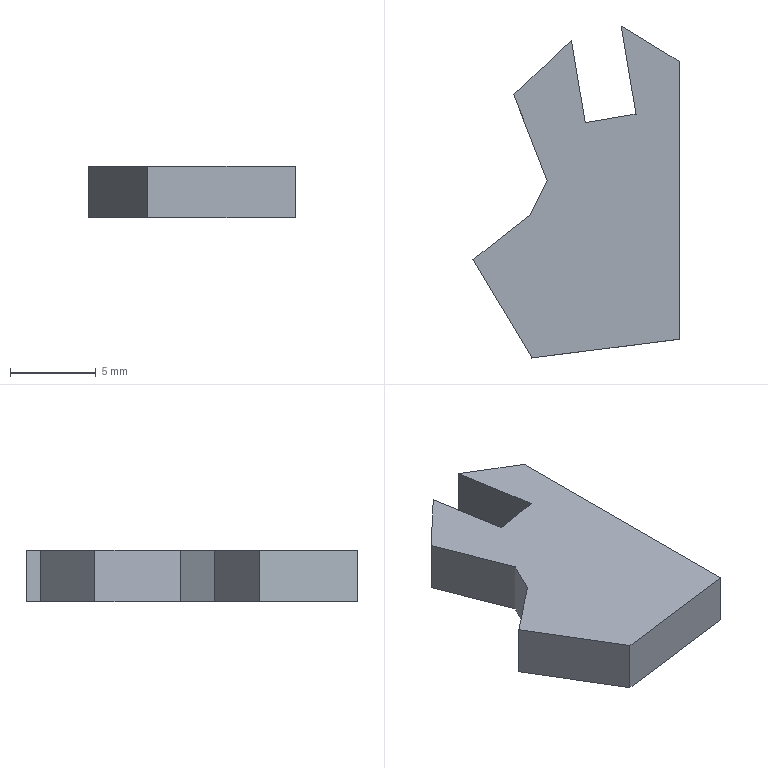Part | SolidWorks | features BaseBody 1 | 1 solid | 13 faces | box 12.009 x 19.33 x 3 mm | volume 454.514 mm3 | spline 7 | plane 6
STEP:
#1=CARTESIAN_POINT('',(-8.721,-24.916,-1.5));
#2=VERTEX_POINT('',#1);
#3=CARTESIAN_POINT('',(-0.1475,-23.826,-1.5));
#4=VERTEX_POINT('',#3);
#5=CARTESIAN_POINT('',(-8.721,-24.916,-1.5));
#6=CARTESIAN_POINT('',(-5.863,-24.552,-1.5));
#7=CARTESIAN_POINT('',(-3.006,-24.188,-1.5));
#8=CARTESIAN_POINT('',(-0.1475,-23.826,-1.5));
#9=B_SPLINE_CURVE_WITH_KNOTS('',3,(#5,#6,#7,#8),.UNSPECIFIED.,.F.,.F.,(4,4),(0.,0.05556),.UNSPECIFIED.);
#10=EDGE_CURVE('',#2,#4,#9,.T.);
#11=ORIENTED_EDGE('',*,*,#10,.F.);
#12=CARTESIAN_POINT('',(-12.156,-19.203,-1.5));
#13=VERTEX_POINT('',#12);
#14=CARTESIAN_POINT('',(-12.156,-19.203,-1.5));
#15=CARTESIAN_POINT('',(-11.011,-21.106,-1.5));
#16=CARTESIAN_POINT('',(-9.865,-23.01,-1.5));
#17=CARTESIAN_POINT('',(-8.721,-24.916,-1.5));
#18=B_SPLINE_CURVE_WITH_KNOTS('',3,(#14,#15,#16,#17),.UNSPECIFIED.,.F.,.F.,(4,4),(0.05556,0.1111),.UNSPECIFIED.);
#19=EDGE_CURVE('',#13,#2,#18,.T.);
#20=ORIENTED_EDGE('',*,*,#19,.F.);
#21=CARTESIAN_POINT('',(-8.807,-16.561,-1.5));
#22=VERTEX_POINT('',#21);
#23=CARTESIAN_POINT('',(-8.807,-16.561,-1.5));
#24=CARTESIAN_POINT('',(-9.924,-17.443,-1.5));
#25=CARTESIAN_POINT('',(-11.04,-18.323,-1.5));
#26=CARTESIAN_POINT('',(-12.156,-19.203,-1.5));
#27=B_SPLINE_CURVE_WITH_KNOTS('',3,(#23,#24,#25,#26),.UNSPECIFIED.,.F.,.F.,(4,4),(0.1111,0.1667),.UNSPECIFIED.);
#28=EDGE_CURVE('',#22,#13,#27,.T.);
#29=ORIENTED_EDGE('',*,*,#28,.F.);
#30=CARTESIAN_POINT('',(-7.838,-14.581,-1.5));
#31=VERTEX_POINT('',#30);
#32=CARTESIAN_POINT('',(-7.838,-14.581,-1.5));
#33=CARTESIAN_POINT('',(-8.163,-15.241,-1.5));
#34=CARTESIAN_POINT('',(-8.485,-15.903,-1.5));
#35=CARTESIAN_POINT('',(-8.807,-16.561,-1.5));
#36=B_SPLINE_CURVE_WITH_KNOTS('',3,(#32,#33,#34,#35),.UNSPECIFIED.,.F.,.F.,(4,4),(0.1667,0.2222),.UNSPECIFIED.);
#37=EDGE_CURVE('',#31,#22,#36,.T.);
#38=ORIENTED_EDGE('',*,*,#37,.F.);
#39=CARTESIAN_POINT('',(-9.774,-9.593,-1.5));
#40=VERTEX_POINT('',#39);
#41=CARTESIAN_POINT('',(-9.774,-9.593,-1.5));
#42=CARTESIAN_POINT('',(-9.129,-11.256,-1.5));
#43=CARTESIAN_POINT('',(-8.485,-12.919,-1.5));
#44=CARTESIAN_POINT('',(-7.838,-14.581,-1.5));
#45=B_SPLINE_CURVE_WITH_KNOTS('',3,(#41,#42,#43,#44),.UNSPECIFIED.,.F.,.F.,(4,4),(0.2222,0.2778),.UNSPECIFIED.);
#46=EDGE_CURVE('',#40,#31,#45,.T.);
#47=ORIENTED_EDGE('',*,*,#46,.F.);
#48=CARTESIAN_POINT('',(-6.421,-6.413,-1.5));
#49=VERTEX_POINT('',#48);
#50=CARTESIAN_POINT('',(-6.421,-6.413,-1.5));
#51=CARTESIAN_POINT('',(-8.658,-8.533,-1.5));
#52=CARTESIAN_POINT('',(-9.774,-9.593,-1.5));
#53=B_SPLINE_CURVE_WITH_KNOTS('',2,(#50,#51,#52),.UNSPECIFIED.,.F.,.F.,(3,3),(0.2778,0.3333),.UNSPECIFIED.);
#54=EDGE_CURVE('',#49,#40,#53,.T.);
#55=ORIENTED_EDGE('',*,*,#54,.F.);
#56=CARTESIAN_POINT('',(-5.614,-11.211,-1.5));
#57=VERTEX_POINT('',#56);
#58=CARTESIAN_POINT('',(-6.421,-6.413,-1.5));
#59=DIRECTION('',(-0.166,0.9861,0.));
#60=VECTOR('',#59,1000.);
#61=LINE('',#58,#60);
#62=EDGE_CURVE('',#57,#49,#61,.T.);
#63=ORIENTED_EDGE('',*,*,#62,.F.);
#64=CARTESIAN_POINT('',(-2.655,-10.713,-1.5));
#65=VERTEX_POINT('',#64);
#66=CARTESIAN_POINT('',(-2.655,-10.713,-1.5));
#67=DIRECTION('',(-0.9861,-0.166,0.));
#68=VECTOR('',#67,1000.);
#69=LINE('',#66,#68);
#70=EDGE_CURVE('',#65,#57,#69,.T.);
#71=ORIENTED_EDGE('',*,*,#70,.F.);
#72=CARTESIAN_POINT('',(-3.518,-5.585,-1.5));
#73=VERTEX_POINT('',#72);
#74=CARTESIAN_POINT('',(-3.518,-5.585,-1.5));
#75=DIRECTION('',(0.166,-0.9861,0.));
#76=VECTOR('',#75,1000.);
#77=LINE('',#74,#76);
#78=EDGE_CURVE('',#73,#65,#77,.T.);
#79=ORIENTED_EDGE('',*,*,#78,.F.);
#80=CARTESIAN_POINT('',(-0.1475,-7.64,-1.5));
#81=VERTEX_POINT('',#80);
#82=CARTESIAN_POINT('',(-0.1475,-7.64,-1.5));
#83=CARTESIAN_POINT('',(-1.25,-6.968,-1.5));
#84=CARTESIAN_POINT('',(-3.432,-5.638,-1.5));
#85=CARTESIAN_POINT('',(-3.518,-5.585,-1.5));
#86=B_SPLINE_CURVE_WITH_KNOTS('',3,(#82,#83,#84,#85),.UNSPECIFIED.,.F.,.F.,(4,4),(0.8344,0.8889),.UNSPECIFIED.);
#87=EDGE_CURVE('',#81,#73,#86,.T.);
#88=ORIENTED_EDGE('',*,*,#87,.F.);
#89=CARTESIAN_POINT('',(-0.1475,-7.64,-1.5));
#90=DIRECTION('',(0.,1.,0.));
#91=VECTOR('',#90,1000.);
#92=LINE('',#89,#91);
#93=EDGE_CURVE('',#4,#81,#92,.T.);
#94=ORIENTED_EDGE('',*,*,#93,.F.);
#95=EDGE_LOOP('',(#11,#20,#29,#38,#47,#55,#63,#71,#79,#88,#94));
#96=FACE_OUTER_BOUND('',#95,.T.);
#97=CARTESIAN_POINT('',(-4.435,-24.37,-1.5));
#98=DIRECTION('',(0.,0.,-1.));
#99=DIRECTION('',(0.,-1.,0.));
#100=AXIS2_PLACEMENT_3D('',#97,#98,#99);
#101=PLANE('',#100);
#102=ADVANCED_FACE('',(#96),#101,.T.);
#103=CARTESIAN_POINT('',(-8.721,-24.916,1.5));
#104=VERTEX_POINT('',#103);
#105=CARTESIAN_POINT('',(-0.1475,-23.826,1.5));
#106=VERTEX_POINT('',#105);
#107=CARTESIAN_POINT('',(-8.721,-24.916,1.5));
#108=CARTESIAN_POINT('',(-5.863,-24.552,1.5));
#109=CARTESIAN_POINT('',(-3.006,-24.188,1.5));
#110=CARTESIAN_POINT('',(-0.1475,-23.826,1.5));
#111=B_SPLINE_CURVE_WITH_KNOTS('',3,(#107,#108,#109,#110),.UNSPECIFIED.,.F.,.F.,(4,4),(0.,0.05556),.UNSPECIFIED.);
#112=EDGE_CURVE('',#104,#106,#111,.T.);
#113=ORIENTED_EDGE('',*,*,#112,.T.);
#114=CARTESIAN_POINT('',(-0.1475,-7.64,1.5));
#115=VERTEX_POINT('',#114);
#116=CARTESIAN_POINT('',(-0.1475,-7.64,1.5));
#117=DIRECTION('',(0.,1.,0.));
#118=VECTOR('',#117,1000.);
#119=LINE('',#116,#118);
#120=EDGE_CURVE('',#106,#115,#119,.T.);
#121=ORIENTED_EDGE('',*,*,#120,.T.);
#122=CARTESIAN_POINT('',(-3.518,-5.585,1.5));
#123=VERTEX_POINT('',#122);
#124=CARTESIAN_POINT('',(-0.1475,-7.64,1.5));
#125=CARTESIAN_POINT('',(-1.25,-6.968,1.5));
#126=CARTESIAN_POINT('',(-3.432,-5.638,1.5));
#127=CARTESIAN_POINT('',(-3.518,-5.585,1.5));
#128=B_SPLINE_CURVE_WITH_KNOTS('',3,(#124,#125,#126,#127),.UNSPECIFIED.,.F.,.F.,(4,4),(0.8344,0.8889),.UNSPECIFIED.);
#129=EDGE_CURVE('',#115,#123,#128,.T.);
#130=ORIENTED_EDGE('',*,*,#129,.T.);
#131=CARTESIAN_POINT('',(-2.655,-10.713,1.5));
#132=VERTEX_POINT('',#131);
#133=CARTESIAN_POINT('',(-3.518,-5.585,1.5));
#134=DIRECTION('',(0.166,-0.9861,0.));
#135=VECTOR('',#134,1000.);
#136=LINE('',#133,#135);
#137=EDGE_CURVE('',#123,#132,#136,.T.);
#138=ORIENTED_EDGE('',*,*,#137,.T.);
#139=CARTESIAN_POINT('',(-5.614,-11.211,1.5));
#140=VERTEX_POINT('',#139);
#141=CARTESIAN_POINT('',(-2.655,-10.713,1.5));
#142=DIRECTION('',(-0.9861,-0.166,0.));
#143=VECTOR('',#142,1000.);
#144=LINE('',#141,#143);
#145=EDGE_CURVE('',#132,#140,#144,.T.);
#146=ORIENTED_EDGE('',*,*,#145,.T.);
#147=CARTESIAN_POINT('',(-6.421,-6.413,1.5));
#148=VERTEX_POINT('',#147);
#149=CARTESIAN_POINT('',(-6.421,-6.413,1.5));
#150=DIRECTION('',(-0.166,0.9861,0.));
#151=VECTOR('',#150,1000.);
#152=LINE('',#149,#151);
#153=EDGE_CURVE('',#140,#148,#152,.T.);
#154=ORIENTED_EDGE('',*,*,#153,.T.);
#155=CARTESIAN_POINT('',(-9.774,-9.593,1.5));
#156=VERTEX_POINT('',#155);
#157=CARTESIAN_POINT('',(-6.421,-6.413,1.5));
#158=CARTESIAN_POINT('',(-8.658,-8.533,1.5));
#159=CARTESIAN_POINT('',(-9.774,-9.593,1.5));
#160=B_SPLINE_CURVE_WITH_KNOTS('',2,(#157,#158,#159),.UNSPECIFIED.,.F.,.F.,(3,3),(0.2778,0.3333),.UNSPECIFIED.);
#161=EDGE_CURVE('',#148,#156,#160,.T.);
#162=ORIENTED_EDGE('',*,*,#161,.T.);
#163=CARTESIAN_POINT('',(-7.838,-14.581,1.5));
#164=VERTEX_POINT('',#163);
#165=CARTESIAN_POINT('',(-9.774,-9.593,1.5));
#166=CARTESIAN_POINT('',(-9.129,-11.256,1.5));
#167=CARTESIAN_POINT('',(-8.485,-12.919,1.5));
#168=CARTESIAN_POINT('',(-7.838,-14.581,1.5));
#169=B_SPLINE_CURVE_WITH_KNOTS('',3,(#165,#166,#167,#168),.UNSPECIFIED.,.F.,.F.,(4,4),(0.2222,0.2778),.UNSPECIFIED.);
#170=EDGE_CURVE('',#156,#164,#169,.T.);
#171=ORIENTED_EDGE('',*,*,#170,.T.);
#172=CARTESIAN_POINT('',(-8.807,-16.561,1.5));
#173=VERTEX_POINT('',#172);
#174=CARTESIAN_POINT('',(-7.838,-14.581,1.5));
#175=CARTESIAN_POINT('',(-8.163,-15.241,1.5));
#176=CARTESIAN_POINT('',(-8.485,-15.903,1.5));
#177=CARTESIAN_POINT('',(-8.807,-16.561,1.5));
#178=B_SPLINE_CURVE_WITH_KNOTS('',3,(#174,#175,#176,#177),.UNSPECIFIED.,.F.,.F.,(4,4),(0.1667,0.2222),.UNSPECIFIED.);
#179=EDGE_CURVE('',#164,#173,#178,.T.);
#180=ORIENTED_EDGE('',*,*,#179,.T.);
#181=CARTESIAN_POINT('',(-12.156,-19.203,1.5));
#182=VERTEX_POINT('',#181);
#183=CARTESIAN_POINT('',(-8.807,-16.561,1.5));
#184=CARTESIAN_POINT('',(-9.924,-17.443,1.5));
#185=CARTESIAN_POINT('',(-11.04,-18.323,1.5));
#186=CARTESIAN_POINT('',(-12.156,-19.203,1.5));
#187=B_SPLINE_CURVE_WITH_KNOTS('',3,(#183,#184,#185,#186),.UNSPECIFIED.,.F.,.F.,(4,4),(0.1111,0.1667),.UNSPECIFIED.);
#188=EDGE_CURVE('',#173,#182,#187,.T.);
#189=ORIENTED_EDGE('',*,*,#188,.T.);
#190=CARTESIAN_POINT('',(-12.156,-19.203,1.5));
#191=CARTESIAN_POINT('',(-11.011,-21.106,1.5));
#192=CARTESIAN_POINT('',(-9.865,-23.01,1.5));
#193=CARTESIAN_POINT('',(-8.721,-24.916,1.5));
#194=B_SPLINE_CURVE_WITH_KNOTS('',3,(#190,#191,#192,#193),.UNSPECIFIED.,.F.,.F.,(4,4),(0.05556,0.1111),.UNSPECIFIED.);
#195=EDGE_CURVE('',#182,#104,#194,.T.);
#196=ORIENTED_EDGE('',*,*,#195,.T.);
#197=EDGE_LOOP('',(#113,#121,#130,#138,#146,#154,#162,#171,#180,#189,#196));
#198=FACE_OUTER_BOUND('',#197,.T.);
#199=CARTESIAN_POINT('',(-4.435,-24.37,1.5));
#200=DIRECTION('',(0.,0.,-1.));
#201=DIRECTION('',(0.,-1.,0.));
#202=AXIS2_PLACEMENT_3D('',#199,#200,#201);
#203=PLANE('',#202);
#204=ADVANCED_FACE('',(#198),#203,.F.);
#205=ORIENTED_EDGE('',*,*,#19,.T.);
#206=CARTESIAN_POINT('',(-8.721,-24.916,1.5));
#207=DIRECTION('',(0.,0.,-1.));
#208=VECTOR('',#207,1000.);
#209=LINE('',#206,#208);
#210=EDGE_CURVE('',#104,#2,#209,.T.);
#211=ORIENTED_EDGE('',*,*,#210,.F.);
#212=ORIENTED_EDGE('',*,*,#195,.F.);
#213=CARTESIAN_POINT('',(-12.156,-19.203,1.5));
#214=DIRECTION('',(0.,0.,-1.));
#215=VECTOR('',#214,1000.);
#216=LINE('',#213,#215);
#217=EDGE_CURVE('',#182,#13,#216,.T.);
#218=ORIENTED_EDGE('',*,*,#217,.T.);
#219=EDGE_LOOP('',(#205,#211,#212,#218));
#220=FACE_OUTER_BOUND('',#219,.T.);
#221=CARTESIAN_POINT('',(-12.156,-19.203,1.5));
#222=CARTESIAN_POINT('',(-12.156,-19.203,-1.5));
#223=CARTESIAN_POINT('',(-11.011,-21.106,1.5));
#224=CARTESIAN_POINT('',(-11.011,-21.106,-1.5));
#225=CARTESIAN_POINT('',(-9.865,-23.01,1.5));
#226=CARTESIAN_POINT('',(-9.865,-23.01,-1.5));
#227=CARTESIAN_POINT('',(-8.721,-24.916,1.5));
#228=CARTESIAN_POINT('',(-8.721,-24.916,-1.5));
#229=B_SPLINE_SURFACE_WITH_KNOTS('',3,1,((#221,#222),(#223,#224),(#225,#226),(#227,#228)),.UNSPECIFIED.,.F.,.F.,.F.,(4,4),(2,2),(0.05556,0.1111),(0.,1.),.UNSPECIFIED.);
#230=ADVANCED_FACE('',(#220),#229,.F.);
#231=ORIENTED_EDGE('',*,*,#28,.T.);
#232=ORIENTED_EDGE('',*,*,#217,.F.);
#233=ORIENTED_EDGE('',*,*,#188,.F.);
#234=CARTESIAN_POINT('',(-8.807,-16.561,1.5));
#235=DIRECTION('',(0.,0.,-1.));
#236=VECTOR('',#235,1000.);
#237=LINE('',#234,#236);
#238=EDGE_CURVE('',#173,#22,#237,.T.);
#239=ORIENTED_EDGE('',*,*,#238,.T.);
#240=EDGE_LOOP('',(#231,#232,#233,#239));
#241=FACE_OUTER_BOUND('',#240,.T.);
#242=CARTESIAN_POINT('',(-8.807,-16.561,1.5));
#243=CARTESIAN_POINT('',(-8.807,-16.561,-1.5));
#244=CARTESIAN_POINT('',(-9.924,-17.443,1.5));
#245=CARTESIAN_POINT('',(-9.924,-17.443,-1.5));
#246=CARTESIAN_POINT('',(-11.04,-18.323,1.5));
#247=CARTESIAN_POINT('',(-11.04,-18.323,-1.5));
#248=CARTESIAN_POINT('',(-12.156,-19.203,1.5));
#249=CARTESIAN_POINT('',(-12.156,-19.203,-1.5));
#250=B_SPLINE_SURFACE_WITH_KNOTS('',3,1,((#242,#243),(#244,#245),(#246,#247),(#248,#249)),.UNSPECIFIED.,.F.,.F.,.F.,(4,4),(2,2),(0.1111,0.1667),(0.,1.),.UNSPECIFIED.);
#251=ADVANCED_FACE('',(#241),#250,.F.);
#252=ORIENTED_EDGE('',*,*,#37,.T.);
#253=ORIENTED_EDGE('',*,*,#238,.F.);
#254=ORIENTED_EDGE('',*,*,#179,.F.);
#255=CARTESIAN_POINT('',(-7.838,-14.581,1.5));
#256=DIRECTION('',(0.,0.,-1.));
#257=VECTOR('',#256,1000.);
#258=LINE('',#255,#257);
#259=EDGE_CURVE('',#164,#31,#258,.T.);
#260=ORIENTED_EDGE('',*,*,#259,.T.);
#261=EDGE_LOOP('',(#252,#253,#254,#260));
#262=FACE_OUTER_BOUND('',#261,.T.);
#263=CARTESIAN_POINT('',(-7.838,-14.581,1.5));
#264=CARTESIAN_POINT('',(-7.838,-14.581,-1.5));
#265=CARTESIAN_POINT('',(-8.163,-15.241,1.5));
#266=CARTESIAN_POINT('',(-8.163,-15.241,-1.5));
#267=CARTESIAN_POINT('',(-8.485,-15.903,1.5));
#268=CARTESIAN_POINT('',(-8.485,-15.903,-1.5));
#269=CARTESIAN_POINT('',(-8.807,-16.561,1.5));
#270=CARTESIAN_POINT('',(-8.807,-16.561,-1.5));
#271=B_SPLINE_SURFACE_WITH_KNOTS('',3,1,((#263,#264),(#265,#266),(#267,#268),(#269,#270)),.UNSPECIFIED.,.F.,.F.,.F.,(4,4),(2,2),(0.1667,0.2222),(0.,1.),.UNSPECIFIED.);
#272=ADVANCED_FACE('',(#262),#271,.F.);
#273=ORIENTED_EDGE('',*,*,#46,.T.);
#274=ORIENTED_EDGE('',*,*,#259,.F.);
#275=ORIENTED_EDGE('',*,*,#170,.F.);
#276=CARTESIAN_POINT('',(-9.774,-9.593,1.5));
#277=DIRECTION('',(0.,0.,-1.));
#278=VECTOR('',#277,1000.);
#279=LINE('',#276,#278);
#280=EDGE_CURVE('',#156,#40,#279,.T.);
#281=ORIENTED_EDGE('',*,*,#280,.T.);
#282=EDGE_LOOP('',(#273,#274,#275,#281));
#283=FACE_OUTER_BOUND('',#282,.T.);
#284=CARTESIAN_POINT('',(-9.774,-9.593,1.5));
#285=CARTESIAN_POINT('',(-9.774,-9.593,-1.5));
#286=CARTESIAN_POINT('',(-9.129,-11.256,1.5));
#287=CARTESIAN_POINT('',(-9.129,-11.256,-1.5));
#288=CARTESIAN_POINT('',(-8.485,-12.919,1.5));
#289=CARTESIAN_POINT('',(-8.485,-12.919,-1.5));
#290=CARTESIAN_POINT('',(-7.838,-14.581,1.5));
#291=CARTESIAN_POINT('',(-7.838,-14.581,-1.5));
#292=B_SPLINE_SURFACE_WITH_KNOTS('',3,1,((#284,#285),(#286,#287),(#288,#289),(#290,#291)),.UNSPECIFIED.,.F.,.F.,.F.,(4,4),(2,2),(0.2222,0.2778),(0.,1.),.UNSPECIFIED.);
#293=ADVANCED_FACE('',(#283),#292,.F.);
#294=ORIENTED_EDGE('',*,*,#54,.T.);
#295=ORIENTED_EDGE('',*,*,#280,.F.);
#296=ORIENTED_EDGE('',*,*,#161,.F.);
#297=CARTESIAN_POINT('',(-6.421,-6.413,1.5));
#298=DIRECTION('',(0.,0.,-1.));
#299=VECTOR('',#298,1000.);
#300=LINE('',#297,#299);
#301=EDGE_CURVE('',#148,#49,#300,.T.);
#302=ORIENTED_EDGE('',*,*,#301,.T.);
#303=EDGE_LOOP('',(#294,#295,#296,#302));
#304=FACE_OUTER_BOUND('',#303,.T.);
#305=CARTESIAN_POINT('',(-6.421,-6.413,1.5));
#306=CARTESIAN_POINT('',(-6.421,-6.413,-1.5));
#307=CARTESIAN_POINT('',(-8.658,-8.533,1.5));
#308=CARTESIAN_POINT('',(-8.658,-8.533,-1.5));
#309=CARTESIAN_POINT('',(-9.774,-9.593,1.5));
#310=CARTESIAN_POINT('',(-9.774,-9.593,-1.5));
#311=B_SPLINE_SURFACE_WITH_KNOTS('',2,1,((#305,#306),(#307,#308),(#309,#310)),.UNSPECIFIED.,.F.,.F.,.F.,(3,3),(2,2),(0.2778,0.3333),(0.,1.),.UNSPECIFIED.);
#312=ADVANCED_FACE('',(#304),#311,.F.);
#313=ORIENTED_EDGE('',*,*,#62,.T.);
#314=ORIENTED_EDGE('',*,*,#301,.F.);
#315=ORIENTED_EDGE('',*,*,#153,.F.);
#316=CARTESIAN_POINT('',(-5.614,-11.211,1.5));
#317=DIRECTION('',(0.,0.,-1.));
#318=VECTOR('',#317,1000.);
#319=LINE('',#316,#318);
#320=EDGE_CURVE('',#140,#57,#319,.T.);
#321=ORIENTED_EDGE('',*,*,#320,.T.);
#322=EDGE_LOOP('',(#313,#314,#315,#321));
#323=FACE_OUTER_BOUND('',#322,.T.);
#324=CARTESIAN_POINT('',(-6.421,-6.413,1.5));
#325=DIRECTION('',(-0.9861,-0.166,0.));
#326=DIRECTION('',(-0.166,0.9861,0.));
#327=AXIS2_PLACEMENT_3D('',#324,#325,#326);
#328=PLANE('',#327);
#329=ADVANCED_FACE('',(#323),#328,.F.);
#330=ORIENTED_EDGE('',*,*,#70,.T.);
#331=ORIENTED_EDGE('',*,*,#320,.F.);
#332=ORIENTED_EDGE('',*,*,#145,.F.);
#333=CARTESIAN_POINT('',(-2.655,-10.713,1.5));
#334=DIRECTION('',(0.,0.,-1.));
#335=VECTOR('',#334,1000.);
#336=LINE('',#333,#335);
#337=EDGE_CURVE('',#132,#65,#336,.T.);
#338=ORIENTED_EDGE('',*,*,#337,.T.);
#339=EDGE_LOOP('',(#330,#331,#332,#338));
#340=FACE_OUTER_BOUND('',#339,.T.);
#341=CARTESIAN_POINT('',(-2.655,-10.713,1.5));
#342=DIRECTION('',(0.166,-0.9861,0.));
#343=DIRECTION('',(0.,0.,-1.));
#344=AXIS2_PLACEMENT_3D('',#341,#342,#343);
#345=PLANE('',#344);
#346=ADVANCED_FACE('',(#340),#345,.F.);
#347=ORIENTED_EDGE('',*,*,#78,.T.);
#348=ORIENTED_EDGE('',*,*,#337,.F.);
#349=ORIENTED_EDGE('',*,*,#137,.F.);
#350=CARTESIAN_POINT('',(-3.518,-5.585,1.5));
#351=DIRECTION('',(0.,0.,-1.));
#352=VECTOR('',#351,1000.);
#353=LINE('',#350,#352);
#354=EDGE_CURVE('',#123,#73,#353,.T.);
#355=ORIENTED_EDGE('',*,*,#354,.T.);
#356=EDGE_LOOP('',(#347,#348,#349,#355));
#357=FACE_OUTER_BOUND('',#356,.T.);
#358=CARTESIAN_POINT('',(-3.518,-5.585,1.5));
#359=DIRECTION('',(0.9861,0.166,0.));
#360=DIRECTION('',(0.,0.,-1.));
#361=AXIS2_PLACEMENT_3D('',#358,#359,#360);
#362=PLANE('',#361);
#363=ADVANCED_FACE('',(#357),#362,.F.);
#364=ORIENTED_EDGE('',*,*,#87,.T.);
#365=ORIENTED_EDGE('',*,*,#354,.F.);
#366=ORIENTED_EDGE('',*,*,#129,.F.);
#367=CARTESIAN_POINT('',(-0.1475,-7.64,1.5));
#368=DIRECTION('',(0.,0.,-1.));
#369=VECTOR('',#368,1000.);
#370=LINE('',#367,#369);
#371=EDGE_CURVE('',#115,#81,#370,.T.);
#372=ORIENTED_EDGE('',*,*,#371,.T.);
#373=EDGE_LOOP('',(#364,#365,#366,#372));
#374=FACE_OUTER_BOUND('',#373,.T.);
#375=CARTESIAN_POINT('',(-0.1475,-7.64,1.5));
#376=CARTESIAN_POINT('',(-0.1475,-7.64,-1.5));
#377=CARTESIAN_POINT('',(-1.25,-6.968,1.5));
#378=CARTESIAN_POINT('',(-1.25,-6.968,-1.5));
#379=CARTESIAN_POINT('',(-3.432,-5.638,1.5));
#380=CARTESIAN_POINT('',(-3.432,-5.638,-1.5));
#381=CARTESIAN_POINT('',(-3.518,-5.585,1.5));
#382=CARTESIAN_POINT('',(-3.518,-5.585,-1.5));
#383=B_SPLINE_SURFACE_WITH_KNOTS('',3,1,((#375,#376),(#377,#378),(#379,#380),(#381,#382)),.UNSPECIFIED.,.F.,.F.,.F.,(4,4),(2,2),(0.8344,0.8889),(0.,1.),.UNSPECIFIED.);
#384=ADVANCED_FACE('',(#374),#383,.F.);
#385=ORIENTED_EDGE('',*,*,#93,.T.);
#386=ORIENTED_EDGE('',*,*,#371,.F.);
#387=ORIENTED_EDGE('',*,*,#120,.F.);
#388=CARTESIAN_POINT('',(-0.1475,-23.826,1.5));
#389=DIRECTION('',(0.,0.,-1.));
#390=VECTOR('',#389,1000.);
#391=LINE('',#388,#390);
#392=EDGE_CURVE('',#106,#4,#391,.T.);
#393=ORIENTED_EDGE('',*,*,#392,.T.);
#394=EDGE_LOOP('',(#385,#386,#387,#393));
#395=FACE_OUTER_BOUND('',#394,.T.);
#396=CARTESIAN_POINT('',(-0.1475,-7.64,1.5));
#397=DIRECTION('',(-1.,0.,0.));
#398=DIRECTION('',(0.,0.,1.));
#399=AXIS2_PLACEMENT_3D('',#396,#397,#398);
#400=PLANE('',#399);
#401=ADVANCED_FACE('',(#395),#400,.F.);
#402=ORIENTED_EDGE('',*,*,#10,.T.);
#403=ORIENTED_EDGE('',*,*,#392,.F.);
#404=ORIENTED_EDGE('',*,*,#112,.F.);
#405=ORIENTED_EDGE('',*,*,#210,.T.);
#406=EDGE_LOOP('',(#402,#403,#404,#405));
#407=FACE_OUTER_BOUND('',#406,.T.);
#408=CARTESIAN_POINT('',(-8.721,-24.916,1.5));
#409=CARTESIAN_POINT('',(-8.721,-24.916,-1.5));
#410=CARTESIAN_POINT('',(-5.863,-24.552,1.5));
#411=CARTESIAN_POINT('',(-5.863,-24.552,-1.5));
#412=CARTESIAN_POINT('',(-3.006,-24.188,1.5));
#413=CARTESIAN_POINT('',(-3.006,-24.188,-1.5));
#414=CARTESIAN_POINT('',(-0.1475,-23.826,1.5));
#415=CARTESIAN_POINT('',(-0.1475,-23.826,-1.5));
#416=B_SPLINE_SURFACE_WITH_KNOTS('',3,1,((#408,#409),(#410,#411),(#412,#413),(#414,#415)),.UNSPECIFIED.,.F.,.F.,.F.,(4,4),(2,2),(0.,0.05556),(0.,1.),.UNSPECIFIED.);
#417=ADVANCED_FACE('',(#407),#416,.F.);
#418=CLOSED_SHELL('',(#102,#204,#230,#251,#272,#293,#312,#329,#346,#363,#384,#401,#417));
#419=MANIFOLD_SOLID_BREP('',#418);
#420=CARTESIAN_POINT('',(0.,0.,0.));
#421=DIRECTION('',(0.,0.,1.));
#422=DIRECTION('',(1.,0.,0.));
#423=AXIS2_PLACEMENT_3D('',#420,#421,#422);
#424=(LENGTH_UNIT()NAMED_UNIT(*)SI_UNIT(.MILLI.,.METRE.));
#425=UNCERTAINTY_MEASURE_WITH_UNIT(LENGTH_MEASURE(0.00001),#424,'','');
#426=(NAMED_UNIT(*)PLANE_ANGLE_UNIT()SI_UNIT($,.RADIAN.));
#427=(NAMED_UNIT(*)SI_UNIT($,.STERADIAN.)SOLID_ANGLE_UNIT());
#428=(GEOMETRIC_REPRESENTATION_CONTEXT(3)GLOBAL_UNCERTAINTY_ASSIGNED_CONTEXT((#425))GLOBAL_UNIT_ASSIGNED_CONTEXT((#424,#426,#427))REPRESENTATION_CONTEXT('',''));
#429=ADVANCED_BREP_SHAPE_REPRESENTATION('',(#419,#423),#428);